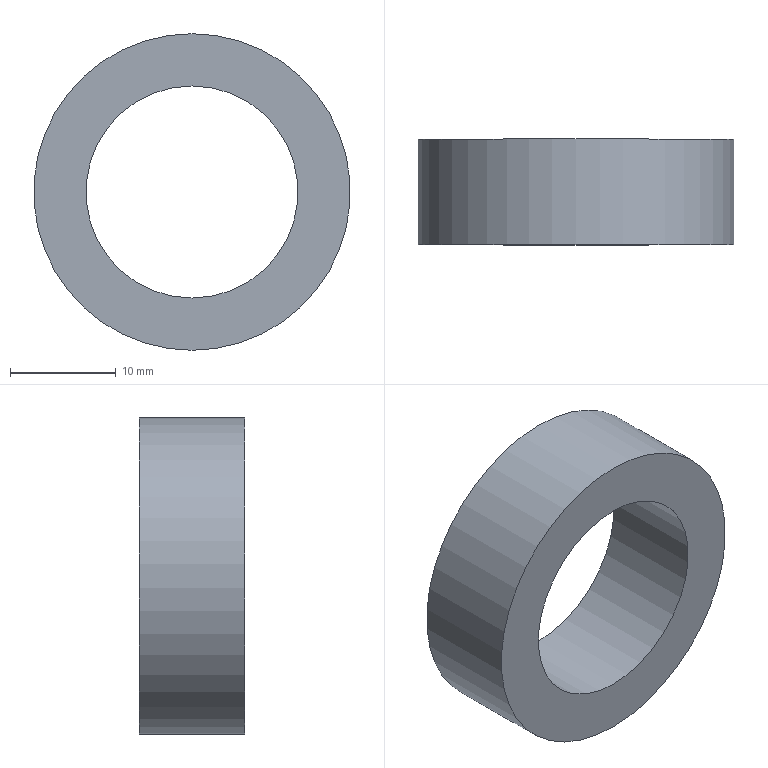Part | STEP file | YBQDJ-YB-24 | 1 solid | 4 faces | box 30 x 10 x 30 mm | volume 3895 mm3 | plane 2 | cylinder 2 | commonest cylinder face diameters 20.1 x1 30 x1
STEP:
#1=CARTESIAN_POINT('',(0.,0.,0.));
#2=DIRECTION('',(0.,0.,1.));
#3=DIRECTION('',(1.,0.,0.));
#4=AXIS2_PLACEMENT_3D('',#1,#2,#3);
#5=CARTESIAN_POINT('',(-183.5,-129.5,93.95));
#6=VERTEX_POINT('',#5);
#7=CARTESIAN_POINT('',(-183.5,-129.5,114.05));
#8=VERTEX_POINT('',#7);
#9=CARTESIAN_POINT('',(-183.5,-129.5,104.));
#10=DIRECTION('',(0.,-1.,0.));
#11=DIRECTION('',(0.,0.,-1.));
#12=AXIS2_PLACEMENT_3D('',#9,#10,#11);
#13=CIRCLE('',#12,10.05);
#14=CARTESIAN_POINT('',(-218.126,-129.5,103.311));
#15=DIRECTION('',(0.,-1.,0.));
#16=DIRECTION('',(1.,0.,0.));
#17=AXIS2_PLACEMENT_3D('',#14,#15,#16);
#18=PLANE('',#17);
#19=CARTESIAN_POINT('',(34.626,0.6886));
#20=DIRECTION('',(0.,-1.));
#21=AXIS2_PLACEMENT_2D('',#19,#20);
#22=CIRCLE('',#21,10.05);
#23=(GEOMETRIC_REPRESENTATION_CONTEXT(2)PARAMETRIC_REPRESENTATION_CONTEXT()REPRESENTATION_CONTEXT('',''));
#24=DEFINITIONAL_REPRESENTATION('',(#22),#23);
#25=PCURVE('',#18,#24);
#26=CARTESIAN_POINT('',(-183.5,-237.3,104.));
#27=DIRECTION('',(0.,1.,0.));
#28=DIRECTION('',(0.,0.,1.));
#29=AXIS2_PLACEMENT_3D('',#26,#27,#28);
#30=CYLINDRICAL_SURFACE('',#29,10.05);
#31=CARTESIAN_POINT('',(3.142,107.8));
#32=DIRECTION('',(-1.,0.));
#33=VECTOR('',#32,1.);
#34=LINE('',#31,#33);
#35=(GEOMETRIC_REPRESENTATION_CONTEXT(2)PARAMETRIC_REPRESENTATION_CONTEXT()REPRESENTATION_CONTEXT('',''));
#36=DEFINITIONAL_REPRESENTATION('',(#34),#35);
#37=PCURVE('',#30,#36);
#38=SURFACE_CURVE('',#13,(#25,#37),.PCURVE_S1.);
#39=EDGE_CURVE('',#6,#8,#38,.T.);
#40=ORIENTED_EDGE('',*,*,#39,.F.);
#41=CARTESIAN_POINT('',(-183.5,-129.5,104.));
#42=DIRECTION('',(0.,-1.,0.));
#43=DIRECTION('',(0.,0.,-1.));
#44=AXIS2_PLACEMENT_3D('',#41,#42,#43);
#45=CIRCLE('',#44,10.05);
#46=CARTESIAN_POINT('',(34.626,0.6886));
#47=DIRECTION('',(0.,-1.));
#48=AXIS2_PLACEMENT_2D('',#46,#47);
#49=CIRCLE('',#48,10.05);
#50=(GEOMETRIC_REPRESENTATION_CONTEXT(2)PARAMETRIC_REPRESENTATION_CONTEXT()REPRESENTATION_CONTEXT('',''));
#51=DEFINITIONAL_REPRESENTATION('',(#49),#50);
#52=PCURVE('',#18,#51);
#53=CARTESIAN_POINT('',(9.425,107.8));
#54=DIRECTION('',(-1.,0.));
#55=VECTOR('',#54,1.);
#56=LINE('',#53,#55);
#57=(GEOMETRIC_REPRESENTATION_CONTEXT(2)PARAMETRIC_REPRESENTATION_CONTEXT()REPRESENTATION_CONTEXT('',''));
#58=DEFINITIONAL_REPRESENTATION('',(#56),#57);
#59=PCURVE('',#30,#58);
#60=SURFACE_CURVE('',#45,(#52,#59),.PCURVE_S1.);
#61=EDGE_CURVE('',#8,#6,#60,.T.);
#62=ORIENTED_EDGE('',*,*,#61,.F.);
#63=EDGE_LOOP('',(#40,#62));
#64=FACE_BOUND('',#63,.T.);
#65=CARTESIAN_POINT('',(-183.5,-129.5,89.));
#66=VERTEX_POINT('',#65);
#67=CARTESIAN_POINT('',(-183.5,-129.5,119.));
#68=VERTEX_POINT('',#67);
#69=CARTESIAN_POINT('',(-183.5,-129.5,104.));
#70=DIRECTION('',(0.,-1.,0.));
#71=DIRECTION('',(0.,0.,-1.));
#72=AXIS2_PLACEMENT_3D('',#69,#70,#71);
#73=CIRCLE('',#72,15.);
#74=CARTESIAN_POINT('',(34.626,0.6886));
#75=DIRECTION('',(0.,-1.));
#76=AXIS2_PLACEMENT_2D('',#74,#75);
#77=CIRCLE('',#76,15.);
#78=(GEOMETRIC_REPRESENTATION_CONTEXT(2)PARAMETRIC_REPRESENTATION_CONTEXT()REPRESENTATION_CONTEXT('',''));
#79=DEFINITIONAL_REPRESENTATION('',(#77),#78);
#80=PCURVE('',#18,#79);
#81=CARTESIAN_POINT('',(-183.5,-237.3,104.));
#82=DIRECTION('',(0.,1.,0.));
#83=DIRECTION('',(0.,0.,1.));
#84=AXIS2_PLACEMENT_3D('',#81,#82,#83);
#85=CYLINDRICAL_SURFACE('',#84,15.);
#86=CARTESIAN_POINT('',(3.142,107.8));
#87=DIRECTION('',(-1.,0.));
#88=VECTOR('',#87,1.);
#89=LINE('',#86,#88);
#90=(GEOMETRIC_REPRESENTATION_CONTEXT(2)PARAMETRIC_REPRESENTATION_CONTEXT()REPRESENTATION_CONTEXT('',''));
#91=DEFINITIONAL_REPRESENTATION('',(#89),#90);
#92=PCURVE('',#85,#91);
#93=SURFACE_CURVE('',#73,(#80,#92),.PCURVE_S1.);
#94=EDGE_CURVE('',#66,#68,#93,.T.);
#95=ORIENTED_EDGE('',*,*,#94,.T.);
#96=CARTESIAN_POINT('',(-183.5,-129.5,104.));
#97=DIRECTION('',(0.,-1.,0.));
#98=DIRECTION('',(0.,0.,-1.));
#99=AXIS2_PLACEMENT_3D('',#96,#97,#98);
#100=CIRCLE('',#99,15.);
#101=CARTESIAN_POINT('',(34.626,0.6886));
#102=DIRECTION('',(0.,-1.));
#103=AXIS2_PLACEMENT_2D('',#101,#102);
#104=CIRCLE('',#103,15.);
#105=(GEOMETRIC_REPRESENTATION_CONTEXT(2)PARAMETRIC_REPRESENTATION_CONTEXT()REPRESENTATION_CONTEXT('',''));
#106=DEFINITIONAL_REPRESENTATION('',(#104),#105);
#107=PCURVE('',#18,#106);
#108=CARTESIAN_POINT('',(9.425,107.8));
#109=DIRECTION('',(-1.,0.));
#110=VECTOR('',#109,1.);
#111=LINE('',#108,#110);
#112=(GEOMETRIC_REPRESENTATION_CONTEXT(2)PARAMETRIC_REPRESENTATION_CONTEXT()REPRESENTATION_CONTEXT('',''));
#113=DEFINITIONAL_REPRESENTATION('',(#111),#112);
#114=PCURVE('',#85,#113);
#115=SURFACE_CURVE('',#100,(#107,#114),.PCURVE_S1.);
#116=EDGE_CURVE('',#68,#66,#115,.T.);
#117=ORIENTED_EDGE('',*,*,#116,.T.);
#118=EDGE_LOOP('',(#95,#117));
#119=FACE_BOUND('',#118,.T.);
#120=ADVANCED_FACE('',(#64,#119),#18,.T.);
#121=CARTESIAN_POINT('',(-183.5,-119.5,119.));
#122=VERTEX_POINT('',#121);
#123=CARTESIAN_POINT('',(-183.5,-119.5,104.));
#124=DIRECTION('',(0.,-1.,0.));
#125=DIRECTION('',(0.,0.,1.));
#126=AXIS2_PLACEMENT_3D('',#123,#124,#125);
#127=CIRCLE('',#126,15.);
#128=CARTESIAN_POINT('',(6.283,117.8));
#129=DIRECTION('',(-1.,0.));
#130=VECTOR('',#129,1.);
#131=LINE('',#128,#130);
#132=(GEOMETRIC_REPRESENTATION_CONTEXT(2)PARAMETRIC_REPRESENTATION_CONTEXT()REPRESENTATION_CONTEXT('',''));
#133=DEFINITIONAL_REPRESENTATION('',(#131),#132);
#134=PCURVE('',#85,#133);
#135=CARTESIAN_POINT('',(-183.5,-119.5,104.));
#136=DIRECTION('',(0.,1.,0.));
#137=DIRECTION('',(0.,0.,1.));
#138=AXIS2_PLACEMENT_3D('',#135,#136,#137);
#139=PLANE('',#138);
#140=CARTESIAN_POINT('',(15.,0.));
#141=CARTESIAN_POINT('',(15.,-25.981));
#142=CARTESIAN_POINT('',(-7.5,-12.99));
#143=CARTESIAN_POINT('',(-30.,0.));
#144=CARTESIAN_POINT('',(-7.5,12.99));
#145=CARTESIAN_POINT('',(15.,25.981));
#146=CARTESIAN_POINT('',(15.,0.));
#147=(BOUNDED_CURVE()B_SPLINE_CURVE(2,(#140,#141,#142,#143,#144,#145,#146),.UNSPECIFIED.,.T.,.F.)B_SPLINE_CURVE_WITH_KNOTS((1,2,2,2,2,1),(-2.094,0.,2.094,4.189,6.283,8.378),.UNSPECIFIED.)CURVE()GEOMETRIC_REPRESENTATION_ITEM()RATIONAL_B_SPLINE_CURVE((1.,0.5,1.,0.5,1.,0.5,1.))REPRESENTATION_ITEM(''));
#148=(GEOMETRIC_REPRESENTATION_CONTEXT(2)PARAMETRIC_REPRESENTATION_CONTEXT()REPRESENTATION_CONTEXT('',''));
#149=DEFINITIONAL_REPRESENTATION('',(#147),#148);
#150=PCURVE('',#139,#149);
#151=SURFACE_CURVE('',#127,(#134,#150),.PCURVE_S1.);
#152=EDGE_CURVE('',#122,#122,#151,.T.);
#153=ORIENTED_EDGE('',*,*,#152,.T.);
#154=CARTESIAN_POINT('',(-183.5,-129.5,119.));
#155=CARTESIAN_POINT('',(-183.5,-119.5,119.));
#156=B_SPLINE_CURVE_WITH_KNOTS('',1,(#154,#155),.UNSPECIFIED.,.F.,.F.,(2,2),(107.8,117.8),.PIECEWISE_BEZIER_KNOTS.);
#157=CARTESIAN_POINT('',(0.,0.));
#158=DIRECTION('',(0.,1.));
#159=VECTOR('',#158,1.);
#160=LINE('',#157,#159);
#161=(GEOMETRIC_REPRESENTATION_CONTEXT(2)PARAMETRIC_REPRESENTATION_CONTEXT()REPRESENTATION_CONTEXT('',''));
#162=DEFINITIONAL_REPRESENTATION('',(#160),#161);
#163=PCURVE('',#85,#162);
#164=CARTESIAN_POINT('',(6.283,0.));
#165=DIRECTION('',(0.,1.));
#166=VECTOR('',#165,1.);
#167=LINE('',#164,#166);
#168=(GEOMETRIC_REPRESENTATION_CONTEXT(2)PARAMETRIC_REPRESENTATION_CONTEXT()REPRESENTATION_CONTEXT('',''));
#169=DEFINITIONAL_REPRESENTATION('',(#167),#168);
#170=PCURVE('',#85,#169);
#171=SEAM_CURVE('',#156,(#163,#170),.PCURVE_S1.);
#172=EDGE_CURVE('',#68,#122,#171,.T.);
#173=ORIENTED_EDGE('',*,*,#172,.F.);
#174=ORIENTED_EDGE('',*,*,#94,.F.);
#175=ORIENTED_EDGE('',*,*,#116,.F.);
#176=ORIENTED_EDGE('',*,*,#172,.T.);
#177=EDGE_LOOP('',(#153,#173,#174,#175,#176));
#178=FACE_BOUND('',#177,.T.);
#179=ADVANCED_FACE('',(#178),#85,.T.);
#180=CARTESIAN_POINT('',(-183.5,-119.5,114.05));
#181=VERTEX_POINT('',#180);
#182=CARTESIAN_POINT('',(-183.5,-119.5,104.));
#183=DIRECTION('',(0.,-1.,0.));
#184=DIRECTION('',(0.,0.,1.));
#185=AXIS2_PLACEMENT_3D('',#182,#183,#184);
#186=CIRCLE('',#185,10.05);
#187=CARTESIAN_POINT('',(6.283,117.8));
#188=DIRECTION('',(-1.,0.));
#189=VECTOR('',#188,1.);
#190=LINE('',#187,#189);
#191=(GEOMETRIC_REPRESENTATION_CONTEXT(2)PARAMETRIC_REPRESENTATION_CONTEXT()REPRESENTATION_CONTEXT('',''));
#192=DEFINITIONAL_REPRESENTATION('',(#190),#191);
#193=PCURVE('',#30,#192);
#194=CARTESIAN_POINT('',(10.05,0.));
#195=CARTESIAN_POINT('',(10.05,-17.407));
#196=CARTESIAN_POINT('',(-5.025,-8.704));
#197=CARTESIAN_POINT('',(-20.1,0.));
#198=CARTESIAN_POINT('',(-5.025,8.704));
#199=CARTESIAN_POINT('',(10.05,17.407));
#200=CARTESIAN_POINT('',(10.05,0.));
#201=(BOUNDED_CURVE()B_SPLINE_CURVE(2,(#194,#195,#196,#197,#198,#199,#200),.UNSPECIFIED.,.T.,.F.)B_SPLINE_CURVE_WITH_KNOTS((1,2,2,2,2,1),(-2.094,0.,2.094,4.189,6.283,8.378),.UNSPECIFIED.)CURVE()GEOMETRIC_REPRESENTATION_ITEM()RATIONAL_B_SPLINE_CURVE((1.,0.5,1.,0.5,1.,0.5,1.))REPRESENTATION_ITEM(''));
#202=(GEOMETRIC_REPRESENTATION_CONTEXT(2)PARAMETRIC_REPRESENTATION_CONTEXT()REPRESENTATION_CONTEXT('',''));
#203=DEFINITIONAL_REPRESENTATION('',(#201),#202);
#204=PCURVE('',#139,#203);
#205=SURFACE_CURVE('',#186,(#193,#204),.PCURVE_S1.);
#206=EDGE_CURVE('',#181,#181,#205,.T.);
#207=ORIENTED_EDGE('',*,*,#206,.T.);
#208=CARTESIAN_POINT('',(-183.5,-129.5,114.05));
#209=CARTESIAN_POINT('',(-183.5,-119.5,114.05));
#210=B_SPLINE_CURVE_WITH_KNOTS('',1,(#208,#209),.UNSPECIFIED.,.F.,.F.,(2,2),(107.8,117.8),.PIECEWISE_BEZIER_KNOTS.);
#211=CARTESIAN_POINT('',(0.,0.));
#212=DIRECTION('',(0.,1.));
#213=VECTOR('',#212,1.);
#214=LINE('',#211,#213);
#215=(GEOMETRIC_REPRESENTATION_CONTEXT(2)PARAMETRIC_REPRESENTATION_CONTEXT()REPRESENTATION_CONTEXT('',''));
#216=DEFINITIONAL_REPRESENTATION('',(#214),#215);
#217=PCURVE('',#30,#216);
#218=CARTESIAN_POINT('',(6.283,0.));
#219=DIRECTION('',(0.,1.));
#220=VECTOR('',#219,1.);
#221=LINE('',#218,#220);
#222=(GEOMETRIC_REPRESENTATION_CONTEXT(2)PARAMETRIC_REPRESENTATION_CONTEXT()REPRESENTATION_CONTEXT('',''));
#223=DEFINITIONAL_REPRESENTATION('',(#221),#222);
#224=PCURVE('',#30,#223);
#225=SEAM_CURVE('',#210,(#217,#224),.PCURVE_S1.);
#226=EDGE_CURVE('',#8,#181,#225,.T.);
#227=ORIENTED_EDGE('',*,*,#226,.F.);
#228=ORIENTED_EDGE('',*,*,#39,.F.);
#229=ORIENTED_EDGE('',*,*,#61,.F.);
#230=ORIENTED_EDGE('',*,*,#226,.T.);
#231=EDGE_LOOP('',(#207,#227,#228,#229,#230));
#232=FACE_BOUND('',#231,.F.);
#233=ADVANCED_FACE('',(#232),#30,.F.);
#234=ORIENTED_EDGE('',*,*,#152,.F.);
#235=EDGE_LOOP('',(#234));
#236=FACE_BOUND('',#235,.T.);
#237=ORIENTED_EDGE('',*,*,#206,.T.);
#238=EDGE_LOOP('',(#237));
#239=FACE_BOUND('',#238,.T.);
#240=ADVANCED_FACE('',(#236,#239),#139,.T.);
#241=CLOSED_SHELL('',(#120,#179,#233,#240));
#242=MANIFOLD_SOLID_BREP('',#241);
#243=(LENGTH_UNIT()NAMED_UNIT(*)SI_UNIT(.MILLI.,.METRE.));
#244=UNCERTAINTY_MEASURE_WITH_UNIT(LENGTH_MEASURE(0.000005),#243,'','');
#245=(NAMED_UNIT(*)PLANE_ANGLE_UNIT()SI_UNIT($,.RADIAN.));
#246=(NAMED_UNIT(*)SI_UNIT($,.STERADIAN.)SOLID_ANGLE_UNIT());
#247=(GEOMETRIC_REPRESENTATION_CONTEXT(3)GLOBAL_UNCERTAINTY_ASSIGNED_CONTEXT((#244))GLOBAL_UNIT_ASSIGNED_CONTEXT((#243,#245,#246))REPRESENTATION_CONTEXT('',''));
#248=ADVANCED_BREP_SHAPE_REPRESENTATION('',(#4,#242),#247);